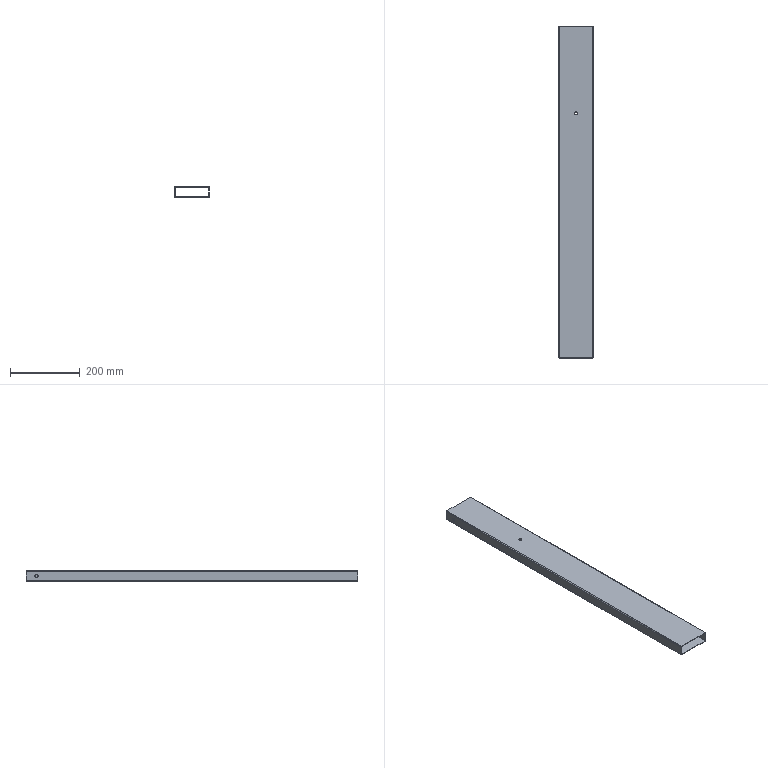Part | STEP file | PN_0071 | 1 solid | 23 faces | box 100 x 950 x 30 mm | volume 355925 mm3 | cylinder 13 | plane 10 | commonest cylinder face diameters 2 x4 5 x4 9 x4 34 x1